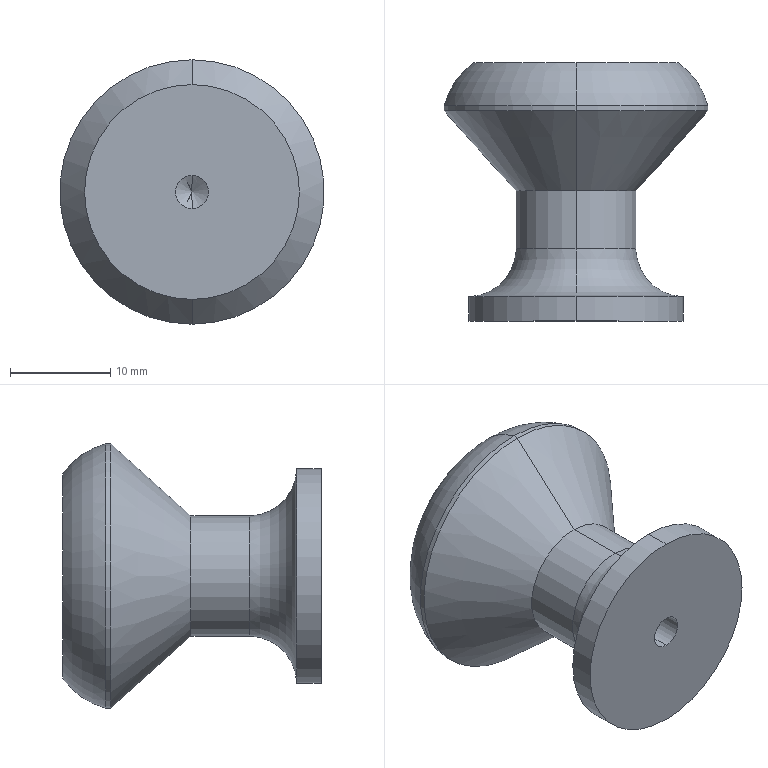Part | SolidWorks | features HoleWzd 1, Revolution 1 | 1 solid | 18 faces | box 26.4 x 25.8 x 26.4 mm | volume 6888 mm3 | cylinder 8 | cone 4 | torus 4 | plane 2 | commonest cylinder face diameters 3.3 x2 12 x2 21.45 x2 26.4 x2
STEP:
#1=CARTESIAN_POINT('',(0.,10.1,1.65));
#2=VERTEX_POINT('',#1);
#3=CARTESIAN_POINT('',(0.,10.1,-1.65));
#4=VERTEX_POINT('',#3);
#5=CARTESIAN_POINT('',(0.,10.1,0.));
#6=DIRECTION('',(0.,-1.,0.));
#7=DIRECTION('',(0.,0.,-1.));
#8=AXIS2_PLACEMENT_3D('',#5,#6,#7);
#9=CIRCLE('',#8,1.65);
#10=EDGE_CURVE('',#2,#4,#9,.T.);
#11=ORIENTED_EDGE('',*,*,#10,.F.);
#12=CARTESIAN_POINT('',(0.,0.,1.65));
#13=VERTEX_POINT('',#12);
#14=CARTESIAN_POINT('',(0.,0.,1.65));
#15=DIRECTION('',(0.,-1.,0.));
#16=VECTOR('',#15,1000.);
#17=LINE('',#14,#16);
#18=EDGE_CURVE('',#2,#13,#17,.T.);
#19=ORIENTED_EDGE('',*,*,#18,.T.);
#20=CARTESIAN_POINT('',(0.,0.,-1.65));
#21=VERTEX_POINT('',#20);
#22=CARTESIAN_POINT('',(0.,0.,0.));
#23=DIRECTION('',(0.,-1.,0.));
#24=DIRECTION('',(0.,0.,-1.));
#25=AXIS2_PLACEMENT_3D('',#22,#23,#24);
#26=CIRCLE('',#25,1.65);
#27=EDGE_CURVE('',#13,#21,#26,.T.);
#28=ORIENTED_EDGE('',*,*,#27,.T.);
#29=CARTESIAN_POINT('',(0.,0.,-1.65));
#30=DIRECTION('',(0.,-1.,0.));
#31=VECTOR('',#30,1000.);
#32=LINE('',#29,#31);
#33=EDGE_CURVE('',#4,#21,#32,.T.);
#34=ORIENTED_EDGE('',*,*,#33,.F.);
#35=EDGE_LOOP('',(#11,#19,#28,#34));
#36=FACE_OUTER_BOUND('',#35,.T.);
#37=CARTESIAN_POINT('',(0.,0.,0.));
#38=DIRECTION('',(0.,-1.,0.));
#39=DIRECTION('',(0.,0.,-1.));
#40=AXIS2_PLACEMENT_3D('',#37,#38,#39);
#41=CYLINDRICAL_SURFACE('',#40,1.65);
#42=ADVANCED_FACE('',(#36),#41,.F.);
#43=CARTESIAN_POINT('',(0.,11.091,0.));
#44=VERTEX_POINT('',#43);
#45=CARTESIAN_POINT('',(0.,10.1,-1.65));
#46=DIRECTION('',(0.,-0.515,-0.8572));
#47=VECTOR('',#46,1000.);
#48=LINE('',#45,#47);
#49=EDGE_CURVE('',#44,#4,#48,.T.);
#50=ORIENTED_EDGE('',*,*,#49,.F.);
#51=CARTESIAN_POINT('',(0.,10.1,1.65));
#52=DIRECTION('',(0.,-0.515,0.8572));
#53=VECTOR('',#52,1000.);
#54=LINE('',#51,#53);
#55=EDGE_CURVE('',#44,#2,#54,.T.);
#56=ORIENTED_EDGE('',*,*,#55,.T.);
#57=ORIENTED_EDGE('',*,*,#10,.T.);
#58=EDGE_LOOP('',(#50,#56,#57));
#59=FACE_OUTER_BOUND('',#58,.T.);
#60=CARTESIAN_POINT('',(0.,10.1,0.));
#61=DIRECTION('',(0.,-1.,0.));
#62=DIRECTION('',(0.,0.,-1.));
#63=AXIS2_PLACEMENT_3D('',#60,#61,#62);
#64=CONICAL_SURFACE('',#63,1.65,1.03);
#65=ADVANCED_FACE('',(#59),#64,.F.);
#66=CARTESIAN_POINT('',(0.,25.8,-10.25));
#67=VERTEX_POINT('',#66);
#68=CARTESIAN_POINT('',(0.,25.8,10.25));
#69=VERTEX_POINT('',#68);
#70=CARTESIAN_POINT('',(0.,25.8,0.));
#71=DIRECTION('',(0.,-1.,0.));
#72=DIRECTION('',(0.,0.,-1.));
#73=AXIS2_PLACEMENT_3D('',#70,#71,#72);
#74=CIRCLE('',#73,10.25);
#75=EDGE_CURVE('',#67,#69,#74,.T.);
#76=ORIENTED_EDGE('',*,*,#75,.T.);
#77=CARTESIAN_POINT('',(0.,21.5,13.2));
#78=VERTEX_POINT('',#77);
#79=CARTESIAN_POINT('',(0.,19.536,5.729));
#80=DIRECTION('',(1.,0.,0.));
#81=DIRECTION('',(0.,0.,-1.));
#82=AXIS2_PLACEMENT_3D('',#79,#80,#81);
#83=CIRCLE('',#82,7.726);
#84=EDGE_CURVE('',#69,#78,#83,.T.);
#85=ORIENTED_EDGE('',*,*,#84,.T.);
#86=CARTESIAN_POINT('',(0.,21.5,-13.2));
#87=VERTEX_POINT('',#86);
#88=CARTESIAN_POINT('',(0.,21.5,0.));
#89=DIRECTION('',(0.,-1.,0.));
#90=DIRECTION('',(0.,0.,-1.));
#91=AXIS2_PLACEMENT_3D('',#88,#89,#90);
#92=CIRCLE('',#91,13.2);
#93=EDGE_CURVE('',#87,#78,#92,.T.);
#94=ORIENTED_EDGE('',*,*,#93,.F.);
#95=CARTESIAN_POINT('',(0.,19.536,-5.729));
#96=DIRECTION('',(-1.,0.,0.));
#97=DIRECTION('',(0.,0.,1.));
#98=AXIS2_PLACEMENT_3D('',#95,#96,#97);
#99=CIRCLE('',#98,7.726);
#100=EDGE_CURVE('',#67,#87,#99,.T.);
#101=ORIENTED_EDGE('',*,*,#100,.F.);
#102=EDGE_LOOP('',(#76,#85,#94,#101));
#103=FACE_OUTER_BOUND('',#102,.T.);
#104=CARTESIAN_POINT('',(0.,19.536,0.));
#105=DIRECTION('',(0.,-1.,0.));
#106=DIRECTION('',(0.,0.,-1.));
#107=AXIS2_PLACEMENT_3D('',#104,#105,#106);
#108=TOROIDAL_SURFACE('',#107,5.729,7.726);
#109=ADVANCED_FACE('',(#103),#108,.T.);
#110=ORIENTED_EDGE('',*,*,#93,.T.);
#111=CARTESIAN_POINT('',(0.,21.,13.2));
#112=VERTEX_POINT('',#111);
#113=CARTESIAN_POINT('',(0.,0.,13.2));
#114=DIRECTION('',(0.,-1.,0.));
#115=VECTOR('',#114,1000.);
#116=LINE('',#113,#115);
#117=EDGE_CURVE('',#78,#112,#116,.T.);
#118=ORIENTED_EDGE('',*,*,#117,.T.);
#119=CARTESIAN_POINT('',(0.,21.,-13.2));
#120=VERTEX_POINT('',#119);
#121=CARTESIAN_POINT('',(0.,21.,0.));
#122=DIRECTION('',(0.,-1.,0.));
#123=DIRECTION('',(0.,0.,-1.));
#124=AXIS2_PLACEMENT_3D('',#121,#122,#123);
#125=CIRCLE('',#124,13.2);
#126=EDGE_CURVE('',#120,#112,#125,.T.);
#127=ORIENTED_EDGE('',*,*,#126,.F.);
#128=CARTESIAN_POINT('',(0.,0.,-13.2));
#129=DIRECTION('',(0.,-1.,0.));
#130=VECTOR('',#129,1000.);
#131=LINE('',#128,#130);
#132=EDGE_CURVE('',#87,#120,#131,.T.);
#133=ORIENTED_EDGE('',*,*,#132,.F.);
#134=EDGE_LOOP('',(#110,#118,#127,#133));
#135=FACE_OUTER_BOUND('',#134,.T.);
#136=CARTESIAN_POINT('',(0.,0.,0.));
#137=DIRECTION('',(0.,-1.,0.));
#138=DIRECTION('',(0.,0.,-1.));
#139=AXIS2_PLACEMENT_3D('',#136,#137,#138);
#140=CYLINDRICAL_SURFACE('',#139,13.2);
#141=ADVANCED_FACE('',(#135),#140,.T.);
#142=CARTESIAN_POINT('',(0.,13.,-6.));
#143=VERTEX_POINT('',#142);
#144=CARTESIAN_POINT('',(0.,13.,6.));
#145=VERTEX_POINT('',#144);
#146=CARTESIAN_POINT('',(0.,13.,0.));
#147=DIRECTION('',(0.,-1.,0.));
#148=DIRECTION('',(0.,0.,-1.));
#149=AXIS2_PLACEMENT_3D('',#146,#147,#148);
#150=CIRCLE('',#149,6.);
#151=EDGE_CURVE('',#143,#145,#150,.T.);
#152=ORIENTED_EDGE('',*,*,#151,.F.);
#153=CARTESIAN_POINT('',(0.,13.,-6.));
#154=DIRECTION('',(0.,0.7433,-0.669));
#155=VECTOR('',#154,1000.);
#156=LINE('',#153,#155);
#157=EDGE_CURVE('',#143,#120,#156,.T.);
#158=ORIENTED_EDGE('',*,*,#157,.T.);
#159=ORIENTED_EDGE('',*,*,#126,.T.);
#160=CARTESIAN_POINT('',(0.,13.,6.));
#161=DIRECTION('',(0.,0.7433,0.669));
#162=VECTOR('',#161,1000.);
#163=LINE('',#160,#162);
#164=EDGE_CURVE('',#145,#112,#163,.T.);
#165=ORIENTED_EDGE('',*,*,#164,.F.);
#166=EDGE_LOOP('',(#152,#158,#159,#165));
#167=FACE_OUTER_BOUND('',#166,.T.);
#168=CARTESIAN_POINT('',(0.,13.,0.));
#169=DIRECTION('',(0.,1.,0.));
#170=DIRECTION('',(0.,0.,1.));
#171=AXIS2_PLACEMENT_3D('',#168,#169,#170);
#172=CONICAL_SURFACE('',#171,6.,0.7328);
#173=ADVANCED_FACE('',(#167),#172,.T.);
#174=ORIENTED_EDGE('',*,*,#151,.T.);
#175=CARTESIAN_POINT('',(0.,7.205,6.));
#176=VERTEX_POINT('',#175);
#177=CARTESIAN_POINT('',(0.,0.,6.));
#178=DIRECTION('',(0.,-1.,0.));
#179=VECTOR('',#178,1000.);
#180=LINE('',#177,#179);
#181=EDGE_CURVE('',#145,#176,#180,.T.);
#182=ORIENTED_EDGE('',*,*,#181,.T.);
#183=CARTESIAN_POINT('',(0.,7.205,-6.));
#184=VERTEX_POINT('',#183);
#185=CARTESIAN_POINT('',(0.,7.205,0.));
#186=DIRECTION('',(0.,-1.,0.));
#187=DIRECTION('',(0.,0.,-1.));
#188=AXIS2_PLACEMENT_3D('',#185,#186,#187);
#189=CIRCLE('',#188,6.);
#190=EDGE_CURVE('',#184,#176,#189,.T.);
#191=ORIENTED_EDGE('',*,*,#190,.F.);
#192=CARTESIAN_POINT('',(0.,0.,-6.));
#193=DIRECTION('',(0.,-1.,0.));
#194=VECTOR('',#193,1000.);
#195=LINE('',#192,#194);
#196=EDGE_CURVE('',#143,#184,#195,.T.);
#197=ORIENTED_EDGE('',*,*,#196,.F.);
#198=EDGE_LOOP('',(#174,#182,#191,#197));
#199=FACE_OUTER_BOUND('',#198,.T.);
#200=CARTESIAN_POINT('',(0.,0.,0.));
#201=DIRECTION('',(0.,-1.,0.));
#202=DIRECTION('',(0.,0.,-1.));
#203=AXIS2_PLACEMENT_3D('',#200,#201,#202);
#204=CYLINDRICAL_SURFACE('',#203,6.);
#205=ADVANCED_FACE('',(#199),#204,.T.);
#206=CARTESIAN_POINT('',(0.,2.45,10.725));
#207=VERTEX_POINT('',#206);
#208=CARTESIAN_POINT('',(0.,2.45,-10.725));
#209=VERTEX_POINT('',#208);
#210=CARTESIAN_POINT('',(0.,2.45,0.));
#211=DIRECTION('',(0.,-1.,0.));
#212=DIRECTION('',(0.,0.,-1.));
#213=AXIS2_PLACEMENT_3D('',#210,#211,#212);
#214=CIRCLE('',#213,10.725);
#215=EDGE_CURVE('',#207,#209,#214,.T.);
#216=ORIENTED_EDGE('',*,*,#215,.F.);
#217=CARTESIAN_POINT('',(0.,7.205,10.755));
#218=DIRECTION('',(1.,0.,0.));
#219=DIRECTION('',(0.,0.,-1.));
#220=AXIS2_PLACEMENT_3D('',#217,#218,#219);
#221=CIRCLE('',#220,4.755);
#222=EDGE_CURVE('',#207,#176,#221,.T.);
#223=ORIENTED_EDGE('',*,*,#222,.T.);
#224=CARTESIAN_POINT('',(0.,7.205,0.));
#225=DIRECTION('',(0.,-1.,0.));
#226=DIRECTION('',(0.,0.,-1.));
#227=AXIS2_PLACEMENT_3D('',#224,#225,#226);
#228=CIRCLE('',#227,6.);
#229=EDGE_CURVE('',#176,#184,#228,.T.);
#230=ORIENTED_EDGE('',*,*,#229,.T.);
#231=CARTESIAN_POINT('',(0.,7.205,-10.755));
#232=DIRECTION('',(-1.,0.,0.));
#233=DIRECTION('',(0.,0.,1.));
#234=AXIS2_PLACEMENT_3D('',#231,#232,#233);
#235=CIRCLE('',#234,4.755);
#236=EDGE_CURVE('',#209,#184,#235,.T.);
#237=ORIENTED_EDGE('',*,*,#236,.F.);
#238=EDGE_LOOP('',(#216,#223,#230,#237));
#239=FACE_OUTER_BOUND('',#238,.T.);
#240=CARTESIAN_POINT('',(0.,7.205,0.));
#241=DIRECTION('',(0.,-1.,0.));
#242=DIRECTION('',(0.,0.,-1.));
#243=AXIS2_PLACEMENT_3D('',#240,#241,#242);
#244=TOROIDAL_SURFACE('',#243,10.755,4.755);
#245=ADVANCED_FACE('',(#239),#244,.F.);
#246=CARTESIAN_POINT('',(0.,2.45,0.));
#247=DIRECTION('',(0.,-1.,0.));
#248=DIRECTION('',(0.,0.,-1.));
#249=AXIS2_PLACEMENT_3D('',#246,#247,#248);
#250=CIRCLE('',#249,10.725);
#251=EDGE_CURVE('',#209,#207,#250,.T.);
#252=ORIENTED_EDGE('',*,*,#251,.T.);
#253=CARTESIAN_POINT('',(0.,0.,10.725));
#254=VERTEX_POINT('',#253);
#255=CARTESIAN_POINT('',(0.,0.,10.725));
#256=DIRECTION('',(0.,-1.,0.));
#257=VECTOR('',#256,1000.);
#258=LINE('',#255,#257);
#259=EDGE_CURVE('',#207,#254,#258,.T.);
#260=ORIENTED_EDGE('',*,*,#259,.T.);
#261=CARTESIAN_POINT('',(0.,0.,-10.725));
#262=VERTEX_POINT('',#261);
#263=CARTESIAN_POINT('',(0.,0.,0.));
#264=DIRECTION('',(0.,-1.,0.));
#265=DIRECTION('',(0.,0.,-1.));
#266=AXIS2_PLACEMENT_3D('',#263,#264,#265);
#267=CIRCLE('',#266,10.725);
#268=EDGE_CURVE('',#262,#254,#267,.T.);
#269=ORIENTED_EDGE('',*,*,#268,.F.);
#270=CARTESIAN_POINT('',(0.,0.,-10.725));
#271=DIRECTION('',(0.,-1.,0.));
#272=VECTOR('',#271,1000.);
#273=LINE('',#270,#272);
#274=EDGE_CURVE('',#209,#262,#273,.T.);
#275=ORIENTED_EDGE('',*,*,#274,.F.);
#276=EDGE_LOOP('',(#252,#260,#269,#275));
#277=FACE_OUTER_BOUND('',#276,.T.);
#278=CARTESIAN_POINT('',(0.,0.,0.));
#279=DIRECTION('',(0.,-1.,0.));
#280=DIRECTION('',(0.,0.,-1.));
#281=AXIS2_PLACEMENT_3D('',#278,#279,#280);
#282=CYLINDRICAL_SURFACE('',#281,10.725);
#283=ADVANCED_FACE('',(#277),#282,.T.);
#284=CARTESIAN_POINT('',(0.,0.,0.));
#285=DIRECTION('',(0.,-1.,0.));
#286=DIRECTION('',(0.,0.,-1.));
#287=AXIS2_PLACEMENT_3D('',#284,#285,#286);
#288=CIRCLE('',#287,1.65);
#289=EDGE_CURVE('',#21,#13,#288,.T.);
#290=ORIENTED_EDGE('',*,*,#289,.F.);
#291=ORIENTED_EDGE('',*,*,#27,.F.);
#292=EDGE_LOOP('',(#290,#291));
#293=FACE_BOUND('',#292,.T.);
#294=ORIENTED_EDGE('',*,*,#268,.T.);
#295=CARTESIAN_POINT('',(0.,0.,0.));
#296=DIRECTION('',(0.,-1.,0.));
#297=DIRECTION('',(0.,0.,-1.));
#298=AXIS2_PLACEMENT_3D('',#295,#296,#297);
#299=CIRCLE('',#298,10.725);
#300=EDGE_CURVE('',#254,#262,#299,.T.);
#301=ORIENTED_EDGE('',*,*,#300,.T.);
#302=EDGE_LOOP('',(#294,#301));
#303=FACE_OUTER_BOUND('',#302,.T.);
#304=CARTESIAN_POINT('',(0.,0.,0.));
#305=DIRECTION('',(0.,-1.,0.));
#306=DIRECTION('',(0.,0.,-1.));
#307=AXIS2_PLACEMENT_3D('',#304,#305,#306);
#308=PLANE('',#307);
#309=ADVANCED_FACE('',(#293,#303),#308,.T.);
#310=ORIENTED_EDGE('',*,*,#259,.F.);
#311=ORIENTED_EDGE('',*,*,#215,.T.);
#312=ORIENTED_EDGE('',*,*,#274,.T.);
#313=ORIENTED_EDGE('',*,*,#300,.F.);
#314=EDGE_LOOP('',(#310,#311,#312,#313));
#315=FACE_OUTER_BOUND('',#314,.T.);
#316=CARTESIAN_POINT('',(0.,0.,0.));
#317=DIRECTION('',(0.,-1.,0.));
#318=DIRECTION('',(0.,0.,-1.));
#319=AXIS2_PLACEMENT_3D('',#316,#317,#318);
#320=CYLINDRICAL_SURFACE('',#319,10.725);
#321=ADVANCED_FACE('',(#315),#320,.T.);
#322=ORIENTED_EDGE('',*,*,#222,.F.);
#323=ORIENTED_EDGE('',*,*,#251,.F.);
#324=ORIENTED_EDGE('',*,*,#236,.T.);
#325=ORIENTED_EDGE('',*,*,#190,.T.);
#326=EDGE_LOOP('',(#322,#323,#324,#325));
#327=FACE_OUTER_BOUND('',#326,.T.);
#328=CARTESIAN_POINT('',(0.,7.205,0.));
#329=DIRECTION('',(0.,-1.,0.));
#330=DIRECTION('',(0.,0.,-1.));
#331=AXIS2_PLACEMENT_3D('',#328,#329,#330);
#332=TOROIDAL_SURFACE('',#331,10.755,4.755);
#333=ADVANCED_FACE('',(#327),#332,.F.);
#334=ORIENTED_EDGE('',*,*,#181,.F.);
#335=CARTESIAN_POINT('',(0.,13.,0.));
#336=DIRECTION('',(0.,-1.,0.));
#337=DIRECTION('',(0.,0.,-1.));
#338=AXIS2_PLACEMENT_3D('',#335,#336,#337);
#339=CIRCLE('',#338,6.);
#340=EDGE_CURVE('',#145,#143,#339,.T.);
#341=ORIENTED_EDGE('',*,*,#340,.T.);
#342=ORIENTED_EDGE('',*,*,#196,.T.);
#343=ORIENTED_EDGE('',*,*,#229,.F.);
#344=EDGE_LOOP('',(#334,#341,#342,#343));
#345=FACE_OUTER_BOUND('',#344,.T.);
#346=CARTESIAN_POINT('',(0.,0.,0.));
#347=DIRECTION('',(0.,-1.,0.));
#348=DIRECTION('',(0.,0.,-1.));
#349=AXIS2_PLACEMENT_3D('',#346,#347,#348);
#350=CYLINDRICAL_SURFACE('',#349,6.);
#351=ADVANCED_FACE('',(#345),#350,.T.);
#352=ORIENTED_EDGE('',*,*,#157,.F.);
#353=ORIENTED_EDGE('',*,*,#340,.F.);
#354=ORIENTED_EDGE('',*,*,#164,.T.);
#355=CARTESIAN_POINT('',(0.,21.,0.));
#356=DIRECTION('',(0.,-1.,0.));
#357=DIRECTION('',(0.,0.,-1.));
#358=AXIS2_PLACEMENT_3D('',#355,#356,#357);
#359=CIRCLE('',#358,13.2);
#360=EDGE_CURVE('',#112,#120,#359,.T.);
#361=ORIENTED_EDGE('',*,*,#360,.T.);
#362=EDGE_LOOP('',(#352,#353,#354,#361));
#363=FACE_OUTER_BOUND('',#362,.T.);
#364=CARTESIAN_POINT('',(0.,13.,0.));
#365=DIRECTION('',(0.,1.,0.));
#366=DIRECTION('',(0.,0.,1.));
#367=AXIS2_PLACEMENT_3D('',#364,#365,#366);
#368=CONICAL_SURFACE('',#367,6.,0.7328);
#369=ADVANCED_FACE('',(#363),#368,.T.);
#370=ORIENTED_EDGE('',*,*,#117,.F.);
#371=CARTESIAN_POINT('',(0.,21.5,0.));
#372=DIRECTION('',(0.,-1.,0.));
#373=DIRECTION('',(0.,0.,-1.));
#374=AXIS2_PLACEMENT_3D('',#371,#372,#373);
#375=CIRCLE('',#374,13.2);
#376=EDGE_CURVE('',#78,#87,#375,.T.);
#377=ORIENTED_EDGE('',*,*,#376,.T.);
#378=ORIENTED_EDGE('',*,*,#132,.T.);
#379=ORIENTED_EDGE('',*,*,#360,.F.);
#380=EDGE_LOOP('',(#370,#377,#378,#379));
#381=FACE_OUTER_BOUND('',#380,.T.);
#382=CARTESIAN_POINT('',(0.,0.,0.));
#383=DIRECTION('',(0.,-1.,0.));
#384=DIRECTION('',(0.,0.,-1.));
#385=AXIS2_PLACEMENT_3D('',#382,#383,#384);
#386=CYLINDRICAL_SURFACE('',#385,13.2);
#387=ADVANCED_FACE('',(#381),#386,.T.);
#388=ORIENTED_EDGE('',*,*,#84,.F.);
#389=CARTESIAN_POINT('',(0.,25.8,0.));
#390=DIRECTION('',(0.,-1.,0.));
#391=DIRECTION('',(0.,0.,-1.));
#392=AXIS2_PLACEMENT_3D('',#389,#390,#391);
#393=CIRCLE('',#392,10.25);
#394=EDGE_CURVE('',#69,#67,#393,.T.);
#395=ORIENTED_EDGE('',*,*,#394,.T.);
#396=ORIENTED_EDGE('',*,*,#100,.T.);
#397=ORIENTED_EDGE('',*,*,#376,.F.);
#398=EDGE_LOOP('',(#388,#395,#396,#397));
#399=FACE_OUTER_BOUND('',#398,.T.);
#400=CARTESIAN_POINT('',(0.,19.536,0.));
#401=DIRECTION('',(0.,-1.,0.));
#402=DIRECTION('',(0.,0.,-1.));
#403=AXIS2_PLACEMENT_3D('',#400,#401,#402);
#404=TOROIDAL_SURFACE('',#403,5.729,7.726);
#405=ADVANCED_FACE('',(#399),#404,.T.);
#406=ORIENTED_EDGE('',*,*,#75,.F.);
#407=ORIENTED_EDGE('',*,*,#394,.F.);
#408=EDGE_LOOP('',(#406,#407));
#409=FACE_OUTER_BOUND('',#408,.T.);
#410=CARTESIAN_POINT('',(0.,25.8,0.));
#411=DIRECTION('',(0.,1.,0.));
#412=DIRECTION('',(0.,0.,1.));
#413=AXIS2_PLACEMENT_3D('',#410,#411,#412);
#414=PLANE('',#413);
#415=ADVANCED_FACE('',(#409),#414,.T.);
#416=ORIENTED_EDGE('',*,*,#55,.F.);
#417=ORIENTED_EDGE('',*,*,#49,.T.);
#418=CARTESIAN_POINT('',(0.,10.1,0.));
#419=DIRECTION('',(0.,-1.,0.));
#420=DIRECTION('',(0.,0.,-1.));
#421=AXIS2_PLACEMENT_3D('',#418,#419,#420);
#422=CIRCLE('',#421,1.65);
#423=EDGE_CURVE('',#4,#2,#422,.T.);
#424=ORIENTED_EDGE('',*,*,#423,.T.);
#425=EDGE_LOOP('',(#416,#417,#424));
#426=FACE_OUTER_BOUND('',#425,.T.);
#427=CARTESIAN_POINT('',(0.,10.1,0.));
#428=DIRECTION('',(0.,-1.,0.));
#429=DIRECTION('',(0.,0.,-1.));
#430=AXIS2_PLACEMENT_3D('',#427,#428,#429);
#431=CONICAL_SURFACE('',#430,1.65,1.03);
#432=ADVANCED_FACE('',(#426),#431,.F.);
#433=ORIENTED_EDGE('',*,*,#18,.F.);
#434=ORIENTED_EDGE('',*,*,#423,.F.);
#435=ORIENTED_EDGE('',*,*,#33,.T.);
#436=ORIENTED_EDGE('',*,*,#289,.T.);
#437=EDGE_LOOP('',(#433,#434,#435,#436));
#438=FACE_OUTER_BOUND('',#437,.T.);
#439=CARTESIAN_POINT('',(0.,0.,0.));
#440=DIRECTION('',(0.,-1.,0.));
#441=DIRECTION('',(0.,0.,-1.));
#442=AXIS2_PLACEMENT_3D('',#439,#440,#441);
#443=CYLINDRICAL_SURFACE('',#442,1.65);
#444=ADVANCED_FACE('',(#438),#443,.F.);
#445=CLOSED_SHELL('',(#42,#65,#109,#141,#173,#205,#245,#283,#309,#321,#333,#351,#369,#387,#405,#415,#432,#444));
#446=MANIFOLD_SOLID_BREP('',#445);
#447=CARTESIAN_POINT('',(0.,0.,0.));
#448=DIRECTION('',(0.,0.,1.));
#449=DIRECTION('',(1.,0.,0.));
#450=AXIS2_PLACEMENT_3D('',#447,#448,#449);
#451=(LENGTH_UNIT()NAMED_UNIT(*)SI_UNIT(.MILLI.,.METRE.));
#452=UNCERTAINTY_MEASURE_WITH_UNIT(LENGTH_MEASURE(0.00001),#451,'','');
#453=(NAMED_UNIT(*)PLANE_ANGLE_UNIT()SI_UNIT($,.RADIAN.));
#454=(NAMED_UNIT(*)SI_UNIT($,.STERADIAN.)SOLID_ANGLE_UNIT());
#455=(GEOMETRIC_REPRESENTATION_CONTEXT(3)GLOBAL_UNCERTAINTY_ASSIGNED_CONTEXT((#452))GLOBAL_UNIT_ASSIGNED_CONTEXT((#451,#453,#454))REPRESENTATION_CONTEXT('',''));
#456=ADVANCED_BREP_SHAPE_REPRESENTATION('',(#446,#450),#455);